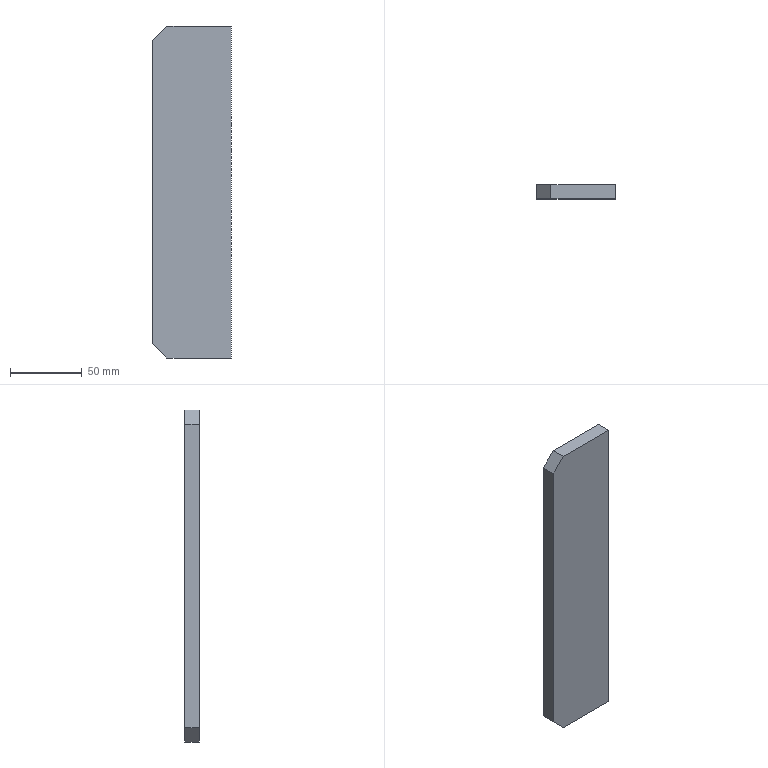Part | STEP file | Beam填充筋Plate-250×125 | 1 solid | 8 faces | box 55 x 10 x 232 mm | volume 126600 mm3 | plane 8
STEP:
#1=CARTESIAN_POINT('',(0.,0.,0.));
#2=DIRECTION('',(0.,0.,1.));
#3=DIRECTION('',(1.,0.,0.));
#4=AXIS2_PLACEMENT_3D('',#1,#2,#3);
#5=CARTESIAN_POINT('',(55.,0.,116.));
#6=VERTEX_POINT('',#5);
#7=CARTESIAN_POINT('',(55.,0.,-116.));
#8=VERTEX_POINT('',#7);
#9=CARTESIAN_POINT('',(55.,0.,-116.));
#10=DIRECTION('',(0.,0.,-1.));
#11=VECTOR('',#10,1.);
#12=LINE('',#9,#11);
#13=CARTESIAN_POINT('',(55.,10.,-116.));
#14=DIRECTION('',(-1.,0.,0.));
#15=DIRECTION('',(0.,0.,1.));
#16=AXIS2_PLACEMENT_3D('',#13,#14,#15);
#17=PLANE('',#16);
#18=CARTESIAN_POINT('',(0.,-10.));
#19=DIRECTION('',(-1.,0.));
#20=VECTOR('',#19,1.);
#21=LINE('',#18,#20);
#22=(GEOMETRIC_REPRESENTATION_CONTEXT(2)PARAMETRIC_REPRESENTATION_CONTEXT()REPRESENTATION_CONTEXT('',''));
#23=DEFINITIONAL_REPRESENTATION('',(#21),#22);
#24=PCURVE('',#17,#23);
#25=CARTESIAN_POINT('',(0.,0.,0.));
#26=DIRECTION('',(0.,-1.,0.));
#27=DIRECTION('',(0.,0.,-1.));
#28=AXIS2_PLACEMENT_3D('',#25,#26,#27);
#29=PLANE('',#28);
#30=CARTESIAN_POINT('',(116.,55.));
#31=DIRECTION('',(1.,0.));
#32=VECTOR('',#31,1.);
#33=LINE('',#30,#32);
#34=(GEOMETRIC_REPRESENTATION_CONTEXT(2)PARAMETRIC_REPRESENTATION_CONTEXT()REPRESENTATION_CONTEXT('',''));
#35=DEFINITIONAL_REPRESENTATION('',(#33),#34);
#36=PCURVE('',#29,#35);
#37=SURFACE_CURVE('',#12,(#24,#36),.PCURVE_S1.);
#38=EDGE_CURVE('',#6,#8,#37,.T.);
#39=ORIENTED_EDGE('',*,*,#38,.T.);
#40=CARTESIAN_POINT('',(55.,10.,-116.));
#41=VERTEX_POINT('',#40);
#42=CARTESIAN_POINT('',(55.,10.,-116.));
#43=DIRECTION('',(0.,-1.,0.));
#44=VECTOR('',#43,1.);
#45=LINE('',#42,#44);
#46=CARTESIAN_POINT('',(0.,0.));
#47=DIRECTION('',(0.,-1.));
#48=VECTOR('',#47,1.);
#49=LINE('',#46,#48);
#50=(GEOMETRIC_REPRESENTATION_CONTEXT(2)PARAMETRIC_REPRESENTATION_CONTEXT()REPRESENTATION_CONTEXT('',''));
#51=DEFINITIONAL_REPRESENTATION('',(#49),#50);
#52=PCURVE('',#17,#51);
#53=CARTESIAN_POINT('',(0.,10.,-116.));
#54=DIRECTION('',(0.,0.,1.));
#55=DIRECTION('',(1.,0.,0.));
#56=AXIS2_PLACEMENT_3D('',#53,#54,#55);
#57=PLANE('',#56);
#58=CARTESIAN_POINT('',(55.,0.));
#59=DIRECTION('',(0.,-1.));
#60=VECTOR('',#59,1.);
#61=LINE('',#58,#60);
#62=(GEOMETRIC_REPRESENTATION_CONTEXT(2)PARAMETRIC_REPRESENTATION_CONTEXT()REPRESENTATION_CONTEXT('',''));
#63=DEFINITIONAL_REPRESENTATION('',(#61),#62);
#64=PCURVE('',#57,#63);
#65=SURFACE_CURVE('',#45,(#52,#64),.PCURVE_S1.);
#66=EDGE_CURVE('',#41,#8,#65,.T.);
#67=ORIENTED_EDGE('',*,*,#66,.F.);
#68=CARTESIAN_POINT('',(55.,10.,116.));
#69=VERTEX_POINT('',#68);
#70=CARTESIAN_POINT('',(55.,10.,-116.));
#71=DIRECTION('',(0.,0.,-1.));
#72=VECTOR('',#71,1.);
#73=LINE('',#70,#72);
#74=CARTESIAN_POINT('',(0.,0.));
#75=DIRECTION('',(-1.,0.));
#76=VECTOR('',#75,1.);
#77=LINE('',#74,#76);
#78=(GEOMETRIC_REPRESENTATION_CONTEXT(2)PARAMETRIC_REPRESENTATION_CONTEXT()REPRESENTATION_CONTEXT('',''));
#79=DEFINITIONAL_REPRESENTATION('',(#77),#78);
#80=PCURVE('',#17,#79);
#81=CARTESIAN_POINT('',(0.,10.,0.));
#82=DIRECTION('',(0.,-1.,0.));
#83=DIRECTION('',(0.,0.,-1.));
#84=AXIS2_PLACEMENT_3D('',#81,#82,#83);
#85=PLANE('',#84);
#86=CARTESIAN_POINT('',(116.,55.));
#87=DIRECTION('',(1.,0.));
#88=VECTOR('',#87,1.);
#89=LINE('',#86,#88);
#90=(GEOMETRIC_REPRESENTATION_CONTEXT(2)PARAMETRIC_REPRESENTATION_CONTEXT()REPRESENTATION_CONTEXT('',''));
#91=DEFINITIONAL_REPRESENTATION('',(#89),#90);
#92=PCURVE('',#85,#91);
#93=SURFACE_CURVE('',#73,(#80,#92),.PCURVE_S1.);
#94=EDGE_CURVE('',#69,#41,#93,.T.);
#95=ORIENTED_EDGE('',*,*,#94,.F.);
#96=CARTESIAN_POINT('',(55.,10.,116.));
#97=DIRECTION('',(0.,-1.,0.));
#98=VECTOR('',#97,1.);
#99=LINE('',#96,#98);
#100=CARTESIAN_POINT('',(232.,0.));
#101=DIRECTION('',(0.,-1.));
#102=VECTOR('',#101,1.);
#103=LINE('',#100,#102);
#104=(GEOMETRIC_REPRESENTATION_CONTEXT(2)PARAMETRIC_REPRESENTATION_CONTEXT()REPRESENTATION_CONTEXT('',''));
#105=DEFINITIONAL_REPRESENTATION('',(#103),#104);
#106=PCURVE('',#17,#105);
#107=CARTESIAN_POINT('',(55.,10.,116.));
#108=DIRECTION('',(0.,0.,-1.));
#109=DIRECTION('',(-1.,0.,0.));
#110=AXIS2_PLACEMENT_3D('',#107,#108,#109);
#111=PLANE('',#110);
#112=CARTESIAN_POINT('',(0.,0.));
#113=DIRECTION('',(0.,-1.));
#114=VECTOR('',#113,1.);
#115=LINE('',#112,#114);
#116=(GEOMETRIC_REPRESENTATION_CONTEXT(2)PARAMETRIC_REPRESENTATION_CONTEXT()REPRESENTATION_CONTEXT('',''));
#117=DEFINITIONAL_REPRESENTATION('',(#115),#116);
#118=PCURVE('',#111,#117);
#119=SURFACE_CURVE('',#99,(#106,#118),.PCURVE_S1.);
#120=EDGE_CURVE('',#69,#6,#119,.T.);
#121=ORIENTED_EDGE('',*,*,#120,.T.);
#122=EDGE_LOOP('',(#39,#67,#95,#121));
#123=FACE_BOUND('',#122,.T.);
#124=ADVANCED_FACE('',(#123),#17,.F.);
#125=CARTESIAN_POINT('',(10.,0.,-116.));
#126=VERTEX_POINT('',#125);
#127=CARTESIAN_POINT('',(0.,0.,-116.));
#128=DIRECTION('',(-1.,0.,0.));
#129=VECTOR('',#128,1.);
#130=LINE('',#127,#129);
#131=CARTESIAN_POINT('',(0.,-10.));
#132=DIRECTION('',(-1.,0.));
#133=VECTOR('',#132,1.);
#134=LINE('',#131,#133);
#135=(GEOMETRIC_REPRESENTATION_CONTEXT(2)PARAMETRIC_REPRESENTATION_CONTEXT()REPRESENTATION_CONTEXT('',''));
#136=DEFINITIONAL_REPRESENTATION('',(#134),#135);
#137=PCURVE('',#57,#136);
#138=CARTESIAN_POINT('',(116.,0.));
#139=DIRECTION('',(0.,-1.));
#140=VECTOR('',#139,1.);
#141=LINE('',#138,#140);
#142=(GEOMETRIC_REPRESENTATION_CONTEXT(2)PARAMETRIC_REPRESENTATION_CONTEXT()REPRESENTATION_CONTEXT('',''));
#143=DEFINITIONAL_REPRESENTATION('',(#141),#142);
#144=PCURVE('',#29,#143);
#145=SURFACE_CURVE('',#130,(#137,#144),.PCURVE_S1.);
#146=EDGE_CURVE('',#8,#126,#145,.T.);
#147=ORIENTED_EDGE('',*,*,#146,.T.);
#148=CARTESIAN_POINT('',(10.,10.,-116.));
#149=VERTEX_POINT('',#148);
#150=CARTESIAN_POINT('',(10.,10.,-116.));
#151=DIRECTION('',(0.,1.,0.));
#152=VECTOR('',#151,1.);
#153=LINE('',#150,#152);
#154=CARTESIAN_POINT('',(10.,0.));
#155=DIRECTION('',(0.,1.));
#156=VECTOR('',#155,1.);
#157=LINE('',#154,#156);
#158=(GEOMETRIC_REPRESENTATION_CONTEXT(2)PARAMETRIC_REPRESENTATION_CONTEXT()REPRESENTATION_CONTEXT('',''));
#159=DEFINITIONAL_REPRESENTATION('',(#157),#158);
#160=PCURVE('',#57,#159);
#161=CARTESIAN_POINT('',(0.,10.,-106.));
#162=DIRECTION('',(0.7071,0.,0.7071));
#163=DIRECTION('',(0.,-1.,0.));
#164=AXIS2_PLACEMENT_3D('',#161,#162,#163);
#165=PLANE('',#164);
#166=CARTESIAN_POINT('',(0.,14.142));
#167=DIRECTION('',(-1.,0.));
#168=VECTOR('',#167,1.);
#169=LINE('',#166,#168);
#170=(GEOMETRIC_REPRESENTATION_CONTEXT(2)PARAMETRIC_REPRESENTATION_CONTEXT()REPRESENTATION_CONTEXT('',''));
#171=DEFINITIONAL_REPRESENTATION('',(#169),#170);
#172=PCURVE('',#165,#171);
#173=SURFACE_CURVE('',#153,(#160,#172),.PCURVE_S1.);
#174=EDGE_CURVE('',#126,#149,#173,.T.);
#175=ORIENTED_EDGE('',*,*,#174,.T.);
#176=CARTESIAN_POINT('',(0.,10.,-116.));
#177=DIRECTION('',(-1.,0.,0.));
#178=VECTOR('',#177,1.);
#179=LINE('',#176,#178);
#180=CARTESIAN_POINT('',(0.,0.));
#181=DIRECTION('',(-1.,0.));
#182=VECTOR('',#181,1.);
#183=LINE('',#180,#182);
#184=(GEOMETRIC_REPRESENTATION_CONTEXT(2)PARAMETRIC_REPRESENTATION_CONTEXT()REPRESENTATION_CONTEXT('',''));
#185=DEFINITIONAL_REPRESENTATION('',(#183),#184);
#186=PCURVE('',#57,#185);
#187=CARTESIAN_POINT('',(116.,0.));
#188=DIRECTION('',(0.,-1.));
#189=VECTOR('',#188,1.);
#190=LINE('',#187,#189);
#191=(GEOMETRIC_REPRESENTATION_CONTEXT(2)PARAMETRIC_REPRESENTATION_CONTEXT()REPRESENTATION_CONTEXT('',''));
#192=DEFINITIONAL_REPRESENTATION('',(#190),#191);
#193=PCURVE('',#85,#192);
#194=SURFACE_CURVE('',#179,(#186,#193),.PCURVE_S1.);
#195=EDGE_CURVE('',#41,#149,#194,.T.);
#196=ORIENTED_EDGE('',*,*,#195,.F.);
#197=ORIENTED_EDGE('',*,*,#66,.T.);
#198=EDGE_LOOP('',(#147,#175,#196,#197));
#199=FACE_BOUND('',#198,.T.);
#200=ADVANCED_FACE('',(#199),#57,.F.);
#201=CARTESIAN_POINT('',(0.,0.,-106.));
#202=VERTEX_POINT('',#201);
#203=CARTESIAN_POINT('',(0.,0.,106.));
#204=VERTEX_POINT('',#203);
#205=CARTESIAN_POINT('',(0.,0.,116.));
#206=DIRECTION('',(0.,0.,1.));
#207=VECTOR('',#206,1.);
#208=LINE('',#205,#207);
#209=CARTESIAN_POINT('',(0.,10.,116.));
#210=DIRECTION('',(1.,0.,0.));
#211=DIRECTION('',(0.,0.,-1.));
#212=AXIS2_PLACEMENT_3D('',#209,#210,#211);
#213=PLANE('',#212);
#214=CARTESIAN_POINT('',(0.,-10.));
#215=DIRECTION('',(-1.,0.));
#216=VECTOR('',#215,1.);
#217=LINE('',#214,#216);
#218=(GEOMETRIC_REPRESENTATION_CONTEXT(2)PARAMETRIC_REPRESENTATION_CONTEXT()REPRESENTATION_CONTEXT('',''));
#219=DEFINITIONAL_REPRESENTATION('',(#217),#218);
#220=PCURVE('',#213,#219);
#221=CARTESIAN_POINT('',(-116.,0.));
#222=DIRECTION('',(-1.,0.));
#223=VECTOR('',#222,1.);
#224=LINE('',#221,#223);
#225=(GEOMETRIC_REPRESENTATION_CONTEXT(2)PARAMETRIC_REPRESENTATION_CONTEXT()REPRESENTATION_CONTEXT('',''));
#226=DEFINITIONAL_REPRESENTATION('',(#224),#225);
#227=PCURVE('',#29,#226);
#228=SURFACE_CURVE('',#208,(#220,#227),.PCURVE_S1.);
#229=EDGE_CURVE('',#202,#204,#228,.T.);
#230=ORIENTED_EDGE('',*,*,#229,.T.);
#231=CARTESIAN_POINT('',(0.,10.,106.));
#232=VERTEX_POINT('',#231);
#233=CARTESIAN_POINT('',(0.,10.,106.));
#234=DIRECTION('',(0.,1.,0.));
#235=VECTOR('',#234,1.);
#236=LINE('',#233,#235);
#237=CARTESIAN_POINT('',(10.,0.));
#238=DIRECTION('',(0.,1.));
#239=VECTOR('',#238,1.);
#240=LINE('',#237,#239);
#241=(GEOMETRIC_REPRESENTATION_CONTEXT(2)PARAMETRIC_REPRESENTATION_CONTEXT()REPRESENTATION_CONTEXT('',''));
#242=DEFINITIONAL_REPRESENTATION('',(#240),#241);
#243=PCURVE('',#213,#242);
#244=CARTESIAN_POINT('',(10.,10.,116.));
#245=DIRECTION('',(0.7071,0.,-0.7071));
#246=DIRECTION('',(0.,-1.,0.));
#247=AXIS2_PLACEMENT_3D('',#244,#245,#246);
#248=PLANE('',#247);
#249=CARTESIAN_POINT('',(0.,14.142));
#250=DIRECTION('',(-1.,0.));
#251=VECTOR('',#250,1.);
#252=LINE('',#249,#251);
#253=(GEOMETRIC_REPRESENTATION_CONTEXT(2)PARAMETRIC_REPRESENTATION_CONTEXT()REPRESENTATION_CONTEXT('',''));
#254=DEFINITIONAL_REPRESENTATION('',(#252),#253);
#255=PCURVE('',#248,#254);
#256=SURFACE_CURVE('',#236,(#243,#255),.PCURVE_S1.);
#257=EDGE_CURVE('',#204,#232,#256,.T.);
#258=ORIENTED_EDGE('',*,*,#257,.T.);
#259=CARTESIAN_POINT('',(0.,10.,-106.));
#260=VERTEX_POINT('',#259);
#261=CARTESIAN_POINT('',(0.,10.,116.));
#262=DIRECTION('',(0.,0.,1.));
#263=VECTOR('',#262,1.);
#264=LINE('',#261,#263);
#265=CARTESIAN_POINT('',(0.,0.));
#266=DIRECTION('',(-1.,0.));
#267=VECTOR('',#266,1.);
#268=LINE('',#265,#267);
#269=(GEOMETRIC_REPRESENTATION_CONTEXT(2)PARAMETRIC_REPRESENTATION_CONTEXT()REPRESENTATION_CONTEXT('',''));
#270=DEFINITIONAL_REPRESENTATION('',(#268),#269);
#271=PCURVE('',#213,#270);
#272=CARTESIAN_POINT('',(-116.,0.));
#273=DIRECTION('',(-1.,0.));
#274=VECTOR('',#273,1.);
#275=LINE('',#272,#274);
#276=(GEOMETRIC_REPRESENTATION_CONTEXT(2)PARAMETRIC_REPRESENTATION_CONTEXT()REPRESENTATION_CONTEXT('',''));
#277=DEFINITIONAL_REPRESENTATION('',(#275),#276);
#278=PCURVE('',#85,#277);
#279=SURFACE_CURVE('',#264,(#271,#278),.PCURVE_S1.);
#280=EDGE_CURVE('',#260,#232,#279,.T.);
#281=ORIENTED_EDGE('',*,*,#280,.F.);
#282=CARTESIAN_POINT('',(0.,10.,-106.));
#283=DIRECTION('',(0.,-1.,0.));
#284=VECTOR('',#283,1.);
#285=LINE('',#282,#284);
#286=CARTESIAN_POINT('',(222.,0.));
#287=DIRECTION('',(0.,-1.));
#288=VECTOR('',#287,1.);
#289=LINE('',#286,#288);
#290=(GEOMETRIC_REPRESENTATION_CONTEXT(2)PARAMETRIC_REPRESENTATION_CONTEXT()REPRESENTATION_CONTEXT('',''));
#291=DEFINITIONAL_REPRESENTATION('',(#289),#290);
#292=PCURVE('',#213,#291);
#293=CARTESIAN_POINT('',(0.,0.));
#294=DIRECTION('',(1.,0.));
#295=VECTOR('',#294,1.);
#296=LINE('',#293,#295);
#297=(GEOMETRIC_REPRESENTATION_CONTEXT(2)PARAMETRIC_REPRESENTATION_CONTEXT()REPRESENTATION_CONTEXT('',''));
#298=DEFINITIONAL_REPRESENTATION('',(#296),#297);
#299=PCURVE('',#165,#298);
#300=SURFACE_CURVE('',#285,(#292,#299),.PCURVE_S1.);
#301=EDGE_CURVE('',#260,#202,#300,.T.);
#302=ORIENTED_EDGE('',*,*,#301,.T.);
#303=EDGE_LOOP('',(#230,#258,#281,#302));
#304=FACE_BOUND('',#303,.T.);
#305=ADVANCED_FACE('',(#304),#213,.F.);
#306=CARTESIAN_POINT('',(10.,10.,116.));
#307=VERTEX_POINT('',#306);
#308=CARTESIAN_POINT('',(55.,10.,116.));
#309=DIRECTION('',(1.,0.,0.));
#310=VECTOR('',#309,1.);
#311=LINE('',#308,#310);
#312=CARTESIAN_POINT('',(0.,0.));
#313=DIRECTION('',(-1.,0.));
#314=VECTOR('',#313,1.);
#315=LINE('',#312,#314);
#316=(GEOMETRIC_REPRESENTATION_CONTEXT(2)PARAMETRIC_REPRESENTATION_CONTEXT()REPRESENTATION_CONTEXT('',''));
#317=DEFINITIONAL_REPRESENTATION('',(#315),#316);
#318=PCURVE('',#111,#317);
#319=CARTESIAN_POINT('',(-116.,55.));
#320=DIRECTION('',(0.,1.));
#321=VECTOR('',#320,1.);
#322=LINE('',#319,#321);
#323=(GEOMETRIC_REPRESENTATION_CONTEXT(2)PARAMETRIC_REPRESENTATION_CONTEXT()REPRESENTATION_CONTEXT('',''));
#324=DEFINITIONAL_REPRESENTATION('',(#322),#323);
#325=PCURVE('',#85,#324);
#326=SURFACE_CURVE('',#311,(#318,#325),.PCURVE_S1.);
#327=EDGE_CURVE('',#307,#69,#326,.T.);
#328=ORIENTED_EDGE('',*,*,#327,.F.);
#329=CARTESIAN_POINT('',(10.,0.,116.));
#330=VERTEX_POINT('',#329);
#331=CARTESIAN_POINT('',(10.,10.,116.));
#332=DIRECTION('',(0.,-1.,0.));
#333=VECTOR('',#332,1.);
#334=LINE('',#331,#333);
#335=CARTESIAN_POINT('',(45.,0.));
#336=DIRECTION('',(0.,-1.));
#337=VECTOR('',#336,1.);
#338=LINE('',#335,#337);
#339=(GEOMETRIC_REPRESENTATION_CONTEXT(2)PARAMETRIC_REPRESENTATION_CONTEXT()REPRESENTATION_CONTEXT('',''));
#340=DEFINITIONAL_REPRESENTATION('',(#338),#339);
#341=PCURVE('',#111,#340);
#342=CARTESIAN_POINT('',(0.,0.));
#343=DIRECTION('',(1.,0.));
#344=VECTOR('',#343,1.);
#345=LINE('',#342,#344);
#346=(GEOMETRIC_REPRESENTATION_CONTEXT(2)PARAMETRIC_REPRESENTATION_CONTEXT()REPRESENTATION_CONTEXT('',''));
#347=DEFINITIONAL_REPRESENTATION('',(#345),#346);
#348=PCURVE('',#248,#347);
#349=SURFACE_CURVE('',#334,(#341,#348),.PCURVE_S1.);
#350=EDGE_CURVE('',#307,#330,#349,.T.);
#351=ORIENTED_EDGE('',*,*,#350,.T.);
#352=CARTESIAN_POINT('',(55.,0.,116.));
#353=DIRECTION('',(1.,0.,0.));
#354=VECTOR('',#353,1.);
#355=LINE('',#352,#354);
#356=CARTESIAN_POINT('',(0.,-10.));
#357=DIRECTION('',(-1.,0.));
#358=VECTOR('',#357,1.);
#359=LINE('',#356,#358);
#360=(GEOMETRIC_REPRESENTATION_CONTEXT(2)PARAMETRIC_REPRESENTATION_CONTEXT()REPRESENTATION_CONTEXT('',''));
#361=DEFINITIONAL_REPRESENTATION('',(#359),#360);
#362=PCURVE('',#111,#361);
#363=CARTESIAN_POINT('',(-116.,55.));
#364=DIRECTION('',(0.,1.));
#365=VECTOR('',#364,1.);
#366=LINE('',#363,#365);
#367=(GEOMETRIC_REPRESENTATION_CONTEXT(2)PARAMETRIC_REPRESENTATION_CONTEXT()REPRESENTATION_CONTEXT('',''));
#368=DEFINITIONAL_REPRESENTATION('',(#366),#367);
#369=PCURVE('',#29,#368);
#370=SURFACE_CURVE('',#355,(#362,#369),.PCURVE_S1.);
#371=EDGE_CURVE('',#330,#6,#370,.T.);
#372=ORIENTED_EDGE('',*,*,#371,.T.);
#373=ORIENTED_EDGE('',*,*,#120,.F.);
#374=EDGE_LOOP('',(#328,#351,#372,#373));
#375=FACE_BOUND('',#374,.T.);
#376=ADVANCED_FACE('',(#375),#111,.F.);
#377=ORIENTED_EDGE('',*,*,#280,.T.);
#378=CARTESIAN_POINT('',(10.,10.,116.));
#379=DIRECTION('',(0.7071,0.,0.7071));
#380=VECTOR('',#379,1.);
#381=LINE('',#378,#380);
#382=CARTESIAN_POINT('',(-116.,10.));
#383=DIRECTION('',(-0.7071,0.7071));
#384=VECTOR('',#383,1.);
#385=LINE('',#382,#384);
#386=(GEOMETRIC_REPRESENTATION_CONTEXT(2)PARAMETRIC_REPRESENTATION_CONTEXT()REPRESENTATION_CONTEXT('',''));
#387=DEFINITIONAL_REPRESENTATION('',(#385),#386);
#388=PCURVE('',#85,#387);
#389=CARTESIAN_POINT('',(0.,0.));
#390=DIRECTION('',(0.,-1.));
#391=VECTOR('',#390,1.);
#392=LINE('',#389,#391);
#393=(GEOMETRIC_REPRESENTATION_CONTEXT(2)PARAMETRIC_REPRESENTATION_CONTEXT()REPRESENTATION_CONTEXT('',''));
#394=DEFINITIONAL_REPRESENTATION('',(#392),#393);
#395=PCURVE('',#248,#394);
#396=SURFACE_CURVE('',#381,(#388,#395),.PCURVE_S1.);
#397=EDGE_CURVE('',#232,#307,#396,.T.);
#398=ORIENTED_EDGE('',*,*,#397,.T.);
#399=ORIENTED_EDGE('',*,*,#327,.T.);
#400=ORIENTED_EDGE('',*,*,#94,.T.);
#401=ORIENTED_EDGE('',*,*,#195,.T.);
#402=CARTESIAN_POINT('',(0.,10.,-106.));
#403=DIRECTION('',(-0.7071,0.,0.7071));
#404=VECTOR('',#403,1.);
#405=LINE('',#402,#404);
#406=CARTESIAN_POINT('',(106.,0.));
#407=DIRECTION('',(-0.7071,-0.7071));
#408=VECTOR('',#407,1.);
#409=LINE('',#406,#408);
#410=(GEOMETRIC_REPRESENTATION_CONTEXT(2)PARAMETRIC_REPRESENTATION_CONTEXT()REPRESENTATION_CONTEXT('',''));
#411=DEFINITIONAL_REPRESENTATION('',(#409),#410);
#412=PCURVE('',#85,#411);
#413=CARTESIAN_POINT('',(0.,0.));
#414=DIRECTION('',(0.,-1.));
#415=VECTOR('',#414,1.);
#416=LINE('',#413,#415);
#417=(GEOMETRIC_REPRESENTATION_CONTEXT(2)PARAMETRIC_REPRESENTATION_CONTEXT()REPRESENTATION_CONTEXT('',''));
#418=DEFINITIONAL_REPRESENTATION('',(#416),#417);
#419=PCURVE('',#165,#418);
#420=SURFACE_CURVE('',#405,(#412,#419),.PCURVE_S1.);
#421=EDGE_CURVE('',#149,#260,#420,.T.);
#422=ORIENTED_EDGE('',*,*,#421,.T.);
#423=EDGE_LOOP('',(#377,#398,#399,#400,#401,#422));
#424=FACE_BOUND('',#423,.T.);
#425=ADVANCED_FACE('',(#424),#85,.F.);
#426=ORIENTED_EDGE('',*,*,#371,.F.);
#427=CARTESIAN_POINT('',(-53.,0.,53.));
#428=DIRECTION('',(-0.7071,0.,-0.7071));
#429=VECTOR('',#428,1.);
#430=LINE('',#427,#429);
#431=CARTESIAN_POINT('',(-53.,-53.));
#432=DIRECTION('',(0.7071,-0.7071));
#433=VECTOR('',#432,1.);
#434=LINE('',#431,#433);
#435=(GEOMETRIC_REPRESENTATION_CONTEXT(2)PARAMETRIC_REPRESENTATION_CONTEXT()REPRESENTATION_CONTEXT('',''));
#436=DEFINITIONAL_REPRESENTATION('',(#434),#435);
#437=PCURVE('',#29,#436);
#438=CARTESIAN_POINT('',(10.,89.095));
#439=DIRECTION('',(0.,1.));
#440=VECTOR('',#439,1.);
#441=LINE('',#438,#440);
#442=(GEOMETRIC_REPRESENTATION_CONTEXT(2)PARAMETRIC_REPRESENTATION_CONTEXT()REPRESENTATION_CONTEXT('',''));
#443=DEFINITIONAL_REPRESENTATION('',(#441),#442);
#444=PCURVE('',#248,#443);
#445=SURFACE_CURVE('',#430,(#437,#444),.PCURVE_S1.);
#446=EDGE_CURVE('',#330,#204,#445,.T.);
#447=ORIENTED_EDGE('',*,*,#446,.T.);
#448=ORIENTED_EDGE('',*,*,#229,.F.);
#449=CARTESIAN_POINT('',(-53.,0.,-53.));
#450=DIRECTION('',(0.7071,0.,-0.7071));
#451=VECTOR('',#450,1.);
#452=LINE('',#449,#451);
#453=CARTESIAN_POINT('',(53.,-53.));
#454=DIRECTION('',(0.7071,0.7071));
#455=VECTOR('',#454,1.);
#456=LINE('',#453,#455);
#457=(GEOMETRIC_REPRESENTATION_CONTEXT(2)PARAMETRIC_REPRESENTATION_CONTEXT()REPRESENTATION_CONTEXT('',''));
#458=DEFINITIONAL_REPRESENTATION('',(#456),#457);
#459=PCURVE('',#29,#458);
#460=CARTESIAN_POINT('',(10.,-74.953));
#461=DIRECTION('',(0.,1.));
#462=VECTOR('',#461,1.);
#463=LINE('',#460,#462);
#464=(GEOMETRIC_REPRESENTATION_CONTEXT(2)PARAMETRIC_REPRESENTATION_CONTEXT()REPRESENTATION_CONTEXT('',''));
#465=DEFINITIONAL_REPRESENTATION('',(#463),#464);
#466=PCURVE('',#165,#465);
#467=SURFACE_CURVE('',#452,(#459,#466),.PCURVE_S1.);
#468=EDGE_CURVE('',#202,#126,#467,.T.);
#469=ORIENTED_EDGE('',*,*,#468,.T.);
#470=ORIENTED_EDGE('',*,*,#146,.F.);
#471=ORIENTED_EDGE('',*,*,#38,.F.);
#472=EDGE_LOOP('',(#426,#447,#448,#469,#470,#471));
#473=FACE_BOUND('',#472,.T.);
#474=ADVANCED_FACE('',(#473),#29,.T.);
#475=ORIENTED_EDGE('',*,*,#397,.F.);
#476=ORIENTED_EDGE('',*,*,#257,.F.);
#477=ORIENTED_EDGE('',*,*,#446,.F.);
#478=ORIENTED_EDGE('',*,*,#350,.F.);
#479=EDGE_LOOP('',(#475,#476,#477,#478));
#480=FACE_BOUND('',#479,.T.);
#481=ADVANCED_FACE('',(#480),#248,.F.);
#482=ORIENTED_EDGE('',*,*,#421,.F.);
#483=ORIENTED_EDGE('',*,*,#174,.F.);
#484=ORIENTED_EDGE('',*,*,#468,.F.);
#485=ORIENTED_EDGE('',*,*,#301,.F.);
#486=EDGE_LOOP('',(#482,#483,#484,#485));
#487=FACE_BOUND('',#486,.T.);
#488=ADVANCED_FACE('',(#487),#165,.F.);
#489=CLOSED_SHELL('',(#124,#200,#305,#376,#425,#474,#481,#488));
#490=MANIFOLD_SOLID_BREP('',#489);
#491=(LENGTH_UNIT()NAMED_UNIT(*)SI_UNIT(.MILLI.,.METRE.));
#492=UNCERTAINTY_MEASURE_WITH_UNIT(LENGTH_MEASURE(0.0000001),#491,'','');
#493=(NAMED_UNIT(*)PLANE_ANGLE_UNIT()SI_UNIT($,.RADIAN.));
#494=(NAMED_UNIT(*)SI_UNIT($,.STERADIAN.)SOLID_ANGLE_UNIT());
#495=(GEOMETRIC_REPRESENTATION_CONTEXT(3)GLOBAL_UNCERTAINTY_ASSIGNED_CONTEXT((#492))GLOBAL_UNIT_ASSIGNED_CONTEXT((#491,#493,#494))REPRESENTATION_CONTEXT('',''));
#496=ADVANCED_BREP_SHAPE_REPRESENTATION('',(#4,#490),#495);